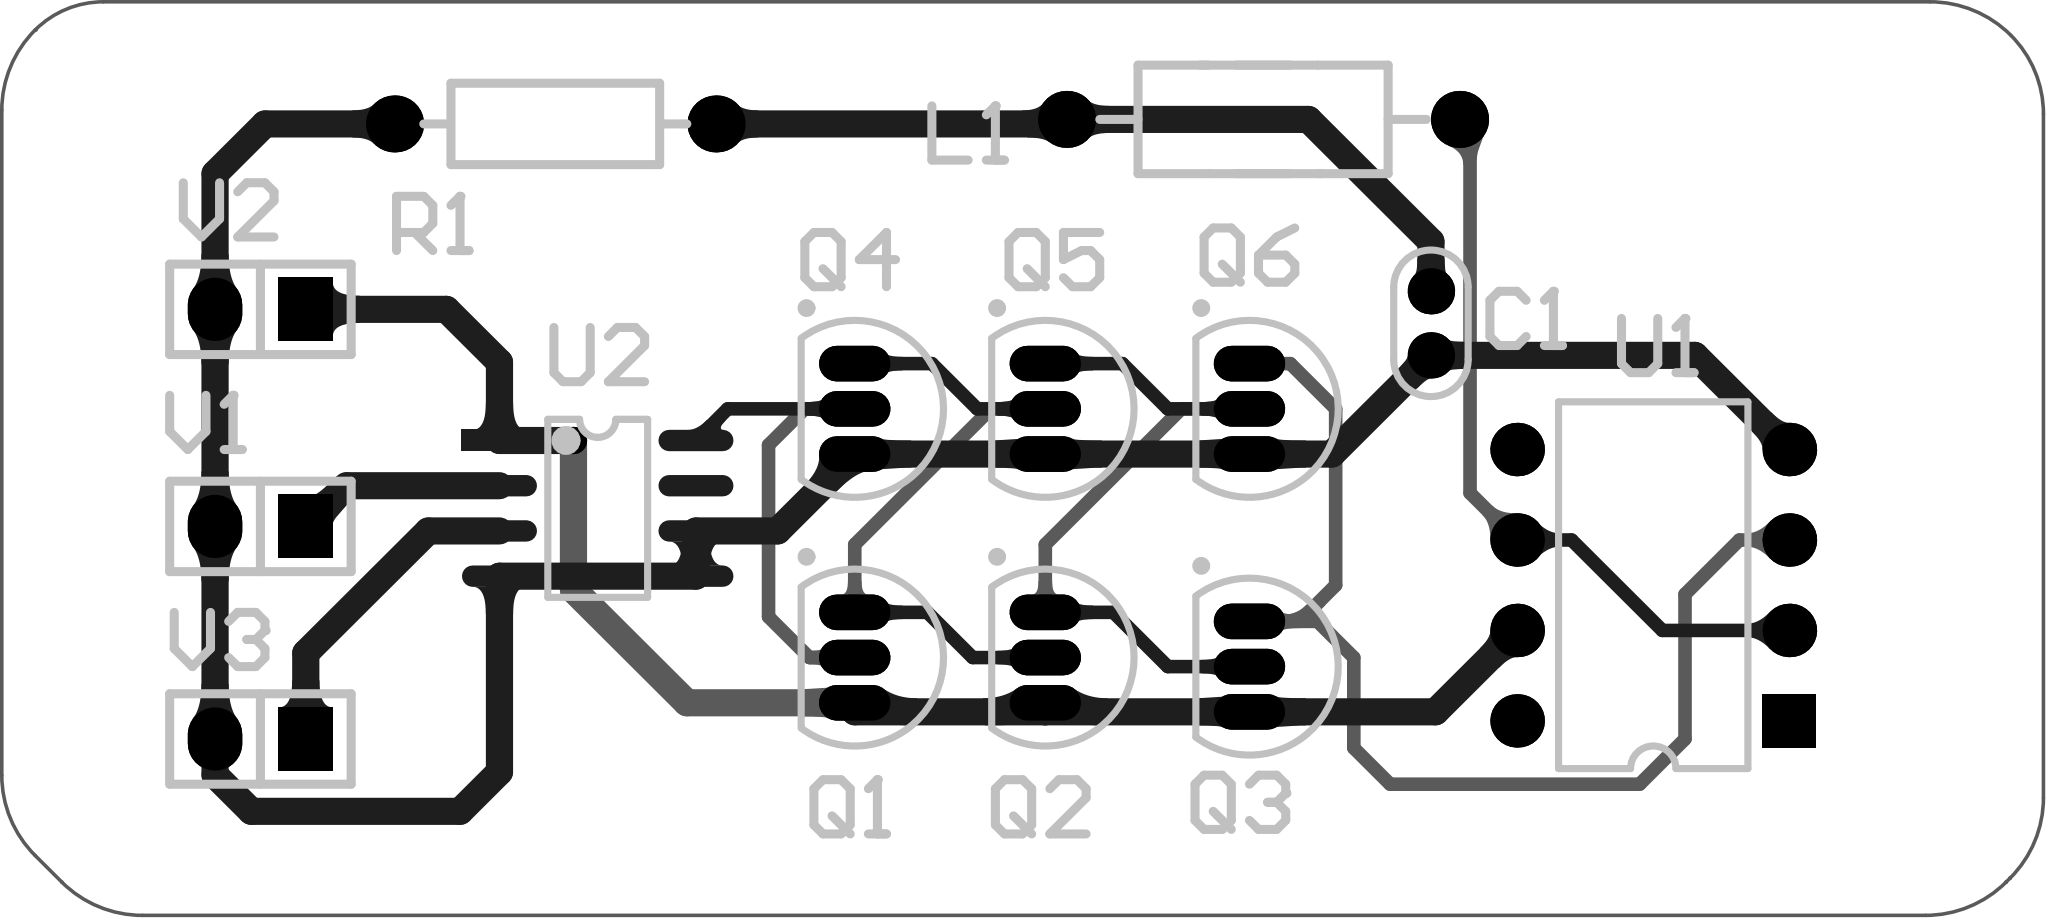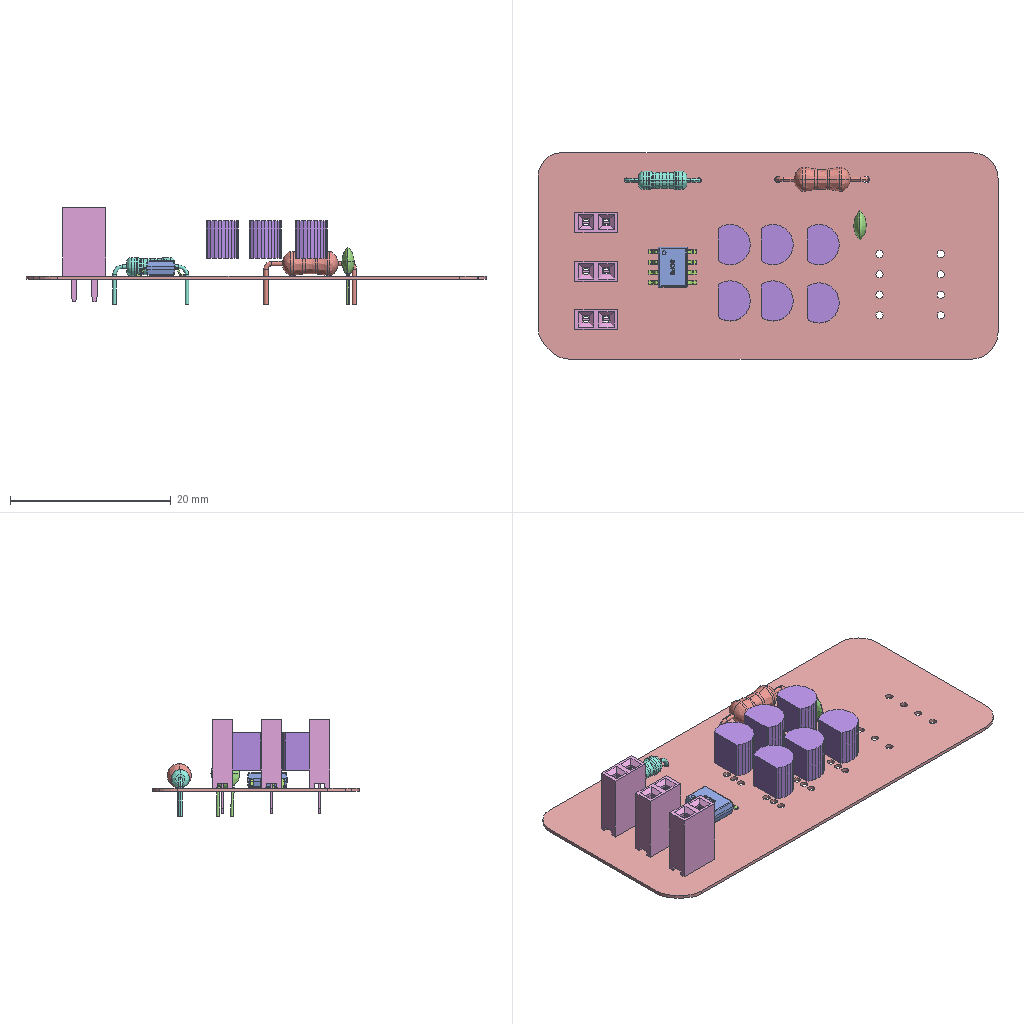Circuit board layout | Altium Designer | box 57.1 x 25.7 x 12 mm
Layer stack:
# Altium Designer layer stack of  (unit mm; dielectric type: 0 none, 1 core, 2 prepreg, 3 surface material)
index,name,kind,layer,copper_thickness_mm,dielectric_type,dielectric_thickness_mm,dielectric_material,dielectric_constant
0,Top Paste,other,,,,,,
1,Top Overlay,other,,,,,,
2,Top Solder,dielectric,,,3,0.0102,Solder Resist,3.5
3,Top Layer,copper,Top Layer,0.0356,,,,
4,Dielectric 1,dielectric,,,0,0.32,FR-4,4.8
5,Bottom Layer,copper,Bottom Layer,0.0356,,,,
6,Bottom Solder,dielectric,,,3,0.0102,Solder Resist,3.5
7,Bottom Overlay,other,,,,,,
8,Bottom Paste,other,,,,,,
# drill layer pairs: low layer,high layer
drill_pair,Top Layer,Bottom Layer
Part placement:
Designator,Comment,Layer,Footprint,Center-X(mm),Center-Y(mm),Rotation
U2,LT1711,TopLayer,SOP8,72.942,67.183,360
V3,Female HDR1X2,TopLayer,Fe-HDR1X2/2.54-S,63.5,60.706,180
V2,Current source,TopLayer,Fe-HDR1X2/2.54-S,63.5,72.771,180
V1,Current source,TopLayer,Fe-HDR1X2/2.54-S,63.5,66.675,180
U1,OP177AZ,TopLayer,Q-8,102.489,65.024,90
R1,47,TopLayer,RS_1/4W,71.755,77.978,360
Q6,2N3906,TopLayer,TO-92A,91.186,69.977,180
Q5,2N3906,TopLayer,TO-92A,85.471,69.977,180
Q4,2N3906,TopLayer,TO-92A,80.137,69.977,180
Q3,2N3904,TopLayer,TO-92A,91.186,62.738,180
Q2,2N3904,TopLayer,TO-92A,85.471,62.992,180
Q1,2N3904,TopLayer,TO-92A,80.137,62.992,180
L1,2.2MH,TopLayer,AL0307,91.567,78.105,180
C1,0.47U,TopLayer,CC_1.8*3.6,96.266,72.379,270
Pad and via stacks:
# Altium Designer via and pad stacks of  (unit mm). Each distinct definition once, with the count of objects using it.
# via: kind,start_layer,end_layer,hole_mm,diameter_mm,mode(0 simple;1 top-mid-bottom;2 full stack),diameter_per_layer,count,example_net
# pad: kind,layer,hole_mm,hole_type(0 round;1 square;2 slot),plating,top_size,top_shape(1 round;2 rect;3 octagon;9 rounded rect),mid_size,bottom_size,mode,footprint,size_per_layer,count,example
pad,Multi-Layer,0.9,0,plated,1.5x1.5,2,1.5x1.5,1.5x1.5,0,Q-8,,1,U1.1
pad,Multi-Layer,0.9,0,plated,1.5x1.5,1,1.5x1.5,1.5x1.5,0,Q-8,,7,U1.2
pad,Multi-Layer,0.9,0,plated,2x1,1,2x1,2x1,0,TO-92A,,18,Q3.3
pad,Multi-Layer,0.8,0,plated,1.6x1.6,1,1.6x1.6,1.6x1.6,0,AL0307,,2,L1.2
pad,Multi-Layer,0.6,0,plated,1.6x1.6,1,1.6x1.6,1.6x1.6,0,RS 1/4W,,2,R1.2
pad,Multi-Layer,0.5,0,plated,1.3x1.3,1,1.3x1.3,1.3x1.3,0,CC 1.8*3.6,,2,C1.2
pad,Multi-Layer,0.8128,0,plated,1.524x1.778,2,1.524x1.778,1.524x1.778,0,Fe-HDR1X2/2.54-S,,3,V3.1
pad,Multi-Layer,0.8128,0,plated,1.524x1.778,1,1.524x1.778,1.524x1.778,0,Fe-HDR1X2/2.54-S,,3,V3.2
pad,Top Layer,0,0,plated,0.6x2.1,1,0.6x2.1,0.6x2.1,0,SOP8,,7,U2.5
pad,Top Layer,0,0,plated,0.6x2.1,2,0.6x2.1,0.6x2.1,0,SOP8,,1,U2.1
via,Top Layer,Bottom Layer,0.381,0.762,0,,1,VCC
Design rules, without the lines most boards share:
# Altium Designer design rules of  (exported by Altium Designer, unit mm)
# columns: name | kind | enabled | priority | scope1 | scope2 | descriptor | typed fields (field=value)
Clearance | 0 | enabled | 1 | All | All | Clearance Constraint (Gap=10mil) (All),(All) | gap=0.254
PlaneConnect | 6 | enabled | 1 | All | All | Power Plane Connect Rule(Relief Connect )(Expansion=20mil) (Conductor Width=10mil) (Air Gap=10mil) (Entries=4) (All) | relief_conductor_width=0.254 relief_entries=4 relief_expansion=0.508
PolygonConnect | 20 | enabled | 1 | All | All | Polygon Connect Rule(Relief Connect )(Conductor Width=10mil) (Relief Angle=90 Angle) (Entries=4) (Air Gap Width=10mil) (All),(All) | connect_style(0=relief,1=direct,2=none)=0 relief_conductor_width=0.254 relief_entries=4
Width | 2 | enabled | 1 | All | All | Width Constraint (Min=10mil) (Max=30mil) (Preferred=10mil) (All) |
RoutingVias | 11 | enabled | 1 | All | All | Routing Via (MinHoleWidth=28mil) (MaxHoleWidth=28mil) (PreferredHoleWidth=28mil) (MinWidth=50mil) (MaxWidth=50mil) (PreferedWidth=50mil) (All) | via_min_hole=0.7112 via_max_hole=0.7112 via_preferred_diameter=1.27 via_preferred_hole=0.7112
PasteMaskExpansion | 14 | enabled | 1 | All | All | Paste Mask Expansion (Expansion =0mil) (All) | expansion=0
SolderMaskExpansion | 13 | enabled | 1 | All | All | Solder Mask Expansion (Expansion =4mil) (All) | expansion=0.1016
DiffPairsRouting | 51 | enabled | 1 | All | All | Differential Pairs Uncoupled Length using the Gap Constraints (Min=10mil) (Max=10mil) (Prefered=10mil)  and Width Constraints (Min=15mil) (Max=15mil) (Prefered=15mil) (All) |
HoleToHoleClearance | 52 | enabled | 1 | All | All | Hole To Hole Clearance (Gap=10mil) (All),(All) | gap=0.254
MinimumSolderMaskSliver | 53 | enabled | 1 | All | All | Minimum Solder Mask Sliver (Gap=0mil) (All),(All) |
SilkToSolderMaskClearance | 54 | enabled | 1 | IsPad | All | Silk To Solder Mask (Clearance=0mil) (IsPad),(All) |
SilkToSilkClearance | 55 | enabled | 1 | All | All | Silk to Silk (Clearance=0mil) (All),(All) |
Classes set for this board:
# Altium Designer classes of  (member kind: 0 net, 1 component, 2 from-to, 3 pad, 4 layer, 5 differential pair, 6 design channel, 7 polygon, 8 structure, 9 xSignal)
# columns: class name | member kind | superclass | members
Sheet1 | 1 | no | C1; L1; Q1; Q2; Q3; Q4; Q5; Q6; R1; U1; U2; V1; V2; V3; U2;